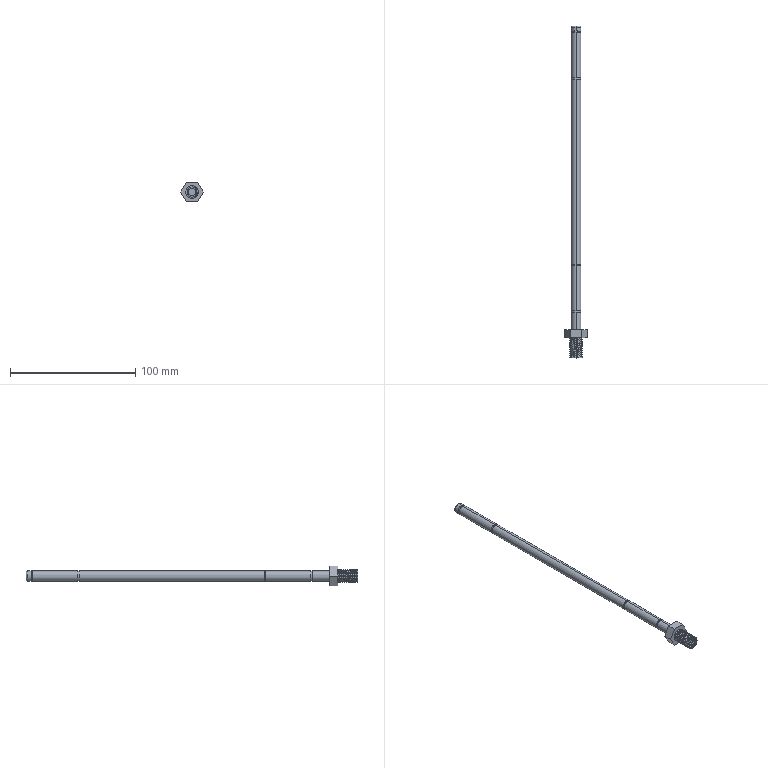Part | SolidWorks | features BaseBody 1 | 1 solid | 94 faces | box 18.244 x 265.5 x 15.8 mm | volume 6663 mm3 | cylinder 67 | plane 22 | spline 3 | torus 2 | commonest cylinder face diameters 10 x23 8.376 x22 8 x12 7.5 x8 6 x2